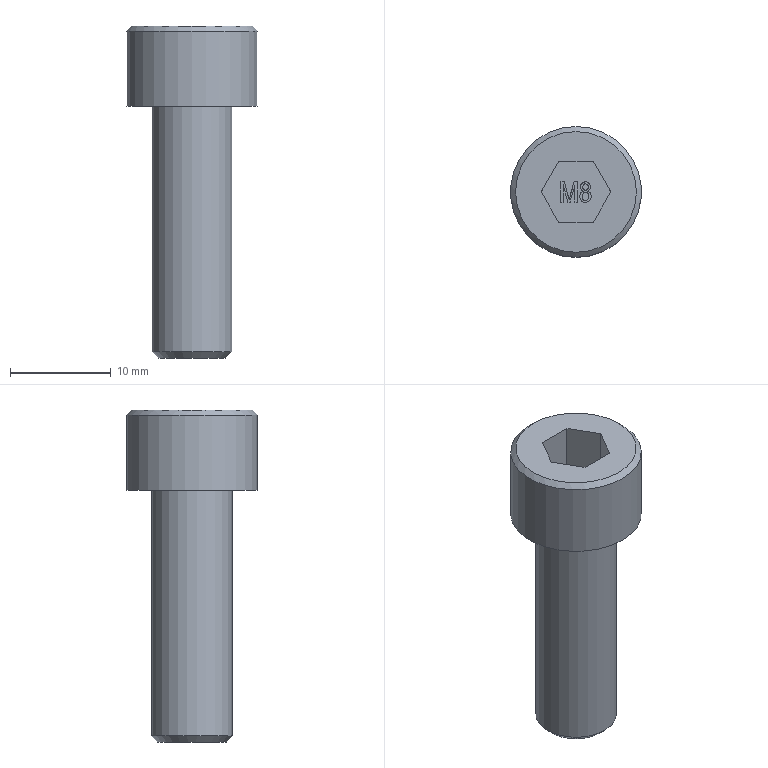Part | STEP file | EM10802500 | 1 solid | 38 faces | box 13 x 13 x 33 mm | volume 2154 mm3 | plane 25 | other 9 | cone 2 | cylinder 2 | commonest cylinder face diameters 8 x1 13 x1